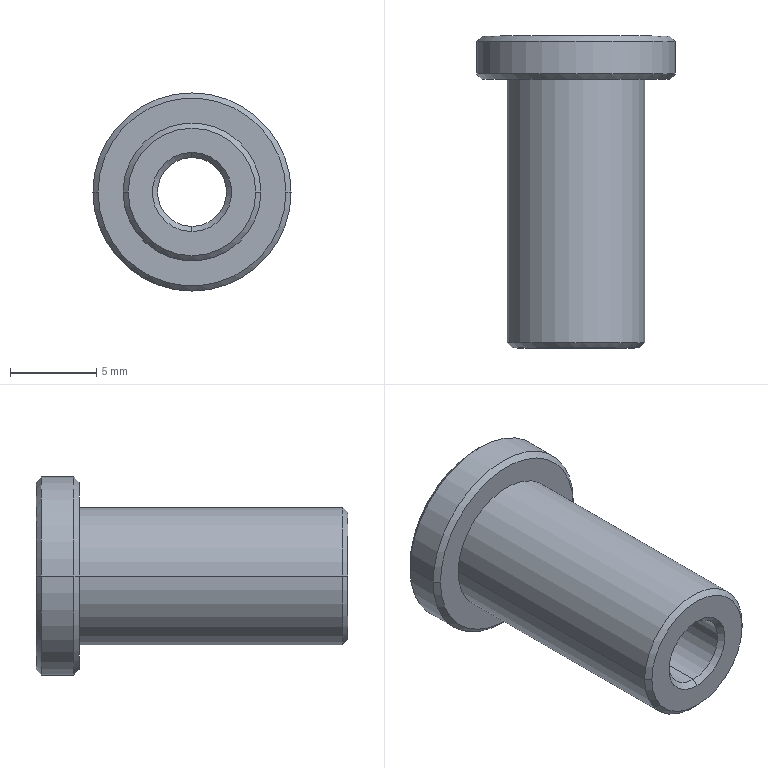Part | STEP file | 1 solid | 19 faces | box 11.5 x 18.1 x 11.5 mm | volume 810.877 mm3 | cone 10 | cylinder 6 | plane 3 | commonest cylinder face diameters 4 x2 8 x2 11.5 x2
STEP:
#1=CARTESIAN_POINT('',(0.,0.,0.));
#2=DIRECTION('',(0.,0.,1.));
#3=DIRECTION('',(1.,0.,0.));
#4=AXIS2_PLACEMENT_3D('',#1,#2,#3);
#5=CARTESIAN_POINT('',(3.7,0.,0.));
#6=VERTEX_POINT('',#5);
#7=CARTESIAN_POINT('',(-3.7,0.,0.));
#8=VERTEX_POINT('',#7);
#9=CARTESIAN_POINT('',(0.,0.,0.));
#10=DIRECTION('',(0.,-1.,0.));
#11=DIRECTION('',(1.,0.,0.));
#12=AXIS2_PLACEMENT_3D('',#9,#10,#11);
#13=CIRCLE('',#12,3.7);
#14=CARTESIAN_POINT('',(0.,0.3,0.));
#15=DIRECTION('',(0.,1.,0.));
#16=DIRECTION('',(-1.,0.,0.));
#17=AXIS2_PLACEMENT_3D('',#14,#15,#16);
#18=CONICAL_SURFACE('',#17,4.,0.7854);
#19=CARTESIAN_POINT('',(3.142,-0.3));
#20=DIRECTION('',(-1.,0.));
#21=VECTOR('',#20,1.);
#22=LINE('',#19,#21);
#23=(GEOMETRIC_REPRESENTATION_CONTEXT(2)PARAMETRIC_REPRESENTATION_CONTEXT()REPRESENTATION_CONTEXT('',''));
#24=DEFINITIONAL_REPRESENTATION('',(#22),#23);
#25=PCURVE('',#18,#24);
#26=CARTESIAN_POINT('',(-4.,0.,0.));
#27=DIRECTION('',(0.,-1.,0.));
#28=DIRECTION('',(1.,0.,0.));
#29=AXIS2_PLACEMENT_3D('',#26,#27,#28);
#30=PLANE('',#29);
#31=CARTESIAN_POINT('',(4.,0.));
#32=DIRECTION('',(1.,0.));
#33=AXIS2_PLACEMENT_2D('',#31,#32);
#34=CIRCLE('',#33,3.7);
#35=(GEOMETRIC_REPRESENTATION_CONTEXT(2)PARAMETRIC_REPRESENTATION_CONTEXT()REPRESENTATION_CONTEXT('',''));
#36=DEFINITIONAL_REPRESENTATION('',(#34),#35);
#37=PCURVE('',#30,#36);
#38=SURFACE_CURVE('',#13,(#25,#37),.PCURVE_S1.);
#39=EDGE_CURVE('',#6,#8,#38,.T.);
#40=ORIENTED_EDGE('',*,*,#39,.F.);
#41=CARTESIAN_POINT('',(4.,0.3,0.));
#42=VERTEX_POINT('',#41);
#43=CARTESIAN_POINT('',(4.,0.3,0.));
#44=DIRECTION('',(0.7071,0.7071,0.));
#45=VECTOR('',#44,1.);
#46=LINE('',#43,#45);
#47=CARTESIAN_POINT('',(3.142,0.));
#48=DIRECTION('',(0.,1.));
#49=VECTOR('',#48,1.);
#50=LINE('',#47,#49);
#51=(GEOMETRIC_REPRESENTATION_CONTEXT(2)PARAMETRIC_REPRESENTATION_CONTEXT()REPRESENTATION_CONTEXT('',''));
#52=DEFINITIONAL_REPRESENTATION('',(#50),#51);
#53=PCURVE('',#18,#52);
#54=CARTESIAN_POINT('',(0.,0.3,0.));
#55=DIRECTION('',(0.,1.,0.));
#56=DIRECTION('',(-1.,0.,0.));
#57=AXIS2_PLACEMENT_3D('',#54,#55,#56);
#58=CONICAL_SURFACE('',#57,4.,0.7854);
#59=CARTESIAN_POINT('',(3.142,0.));
#60=DIRECTION('',(0.,1.));
#61=VECTOR('',#60,1.);
#62=LINE('',#59,#61);
#63=(GEOMETRIC_REPRESENTATION_CONTEXT(2)PARAMETRIC_REPRESENTATION_CONTEXT()REPRESENTATION_CONTEXT('',''));
#64=DEFINITIONAL_REPRESENTATION('',(#62),#63);
#65=PCURVE('',#58,#64);
#66=SURFACE_CURVE('',#46,(#53,#65),.PCURVE_S1.);
#67=EDGE_CURVE('',#6,#42,#66,.T.);
#68=ORIENTED_EDGE('',*,*,#67,.T.);
#69=CARTESIAN_POINT('',(-4.,0.3,0.));
#70=VERTEX_POINT('',#69);
#71=CARTESIAN_POINT('',(0.,0.3,0.));
#72=DIRECTION('',(0.,1.,0.));
#73=DIRECTION('',(1.,0.,0.));
#74=AXIS2_PLACEMENT_3D('',#71,#72,#73);
#75=CIRCLE('',#74,4.);
#76=CARTESIAN_POINT('',(-3.142,0.));
#77=DIRECTION('',(1.,0.));
#78=VECTOR('',#77,1.);
#79=LINE('',#76,#78);
#80=(GEOMETRIC_REPRESENTATION_CONTEXT(2)PARAMETRIC_REPRESENTATION_CONTEXT()REPRESENTATION_CONTEXT('',''));
#81=DEFINITIONAL_REPRESENTATION('',(#79),#80);
#82=PCURVE('',#18,#81);
#83=CARTESIAN_POINT('',(0.,15.6,0.));
#84=DIRECTION('',(0.,1.,0.));
#85=DIRECTION('',(-1.,0.,0.));
#86=AXIS2_PLACEMENT_3D('',#83,#84,#85);
#87=CYLINDRICAL_SURFACE('',#86,4.);
#88=CARTESIAN_POINT('',(-3.142,-15.3));
#89=DIRECTION('',(1.,0.));
#90=VECTOR('',#89,1.);
#91=LINE('',#88,#90);
#92=(GEOMETRIC_REPRESENTATION_CONTEXT(2)PARAMETRIC_REPRESENTATION_CONTEXT()REPRESENTATION_CONTEXT('',''));
#93=DEFINITIONAL_REPRESENTATION('',(#91),#92);
#94=PCURVE('',#87,#93);
#95=SURFACE_CURVE('',#75,(#82,#94),.PCURVE_S1.);
#96=EDGE_CURVE('',#70,#42,#95,.T.);
#97=ORIENTED_EDGE('',*,*,#96,.F.);
#98=CARTESIAN_POINT('',(-4.,0.3,0.));
#99=DIRECTION('',(-0.7071,0.7071,0.));
#100=VECTOR('',#99,1.);
#101=LINE('',#98,#100);
#102=CARTESIAN_POINT('',(0.,0.));
#103=DIRECTION('',(0.,1.));
#104=VECTOR('',#103,1.);
#105=LINE('',#102,#104);
#106=(GEOMETRIC_REPRESENTATION_CONTEXT(2)PARAMETRIC_REPRESENTATION_CONTEXT()REPRESENTATION_CONTEXT('',''));
#107=DEFINITIONAL_REPRESENTATION('',(#105),#106);
#108=PCURVE('',#18,#107);
#109=CARTESIAN_POINT('',(6.283,0.));
#110=DIRECTION('',(0.,1.));
#111=VECTOR('',#110,1.);
#112=LINE('',#109,#111);
#113=(GEOMETRIC_REPRESENTATION_CONTEXT(2)PARAMETRIC_REPRESENTATION_CONTEXT()REPRESENTATION_CONTEXT('',''));
#114=DEFINITIONAL_REPRESENTATION('',(#112),#113);
#115=PCURVE('',#58,#114);
#116=SURFACE_CURVE('',#101,(#108,#115),.PCURVE_S1.);
#117=EDGE_CURVE('',#8,#70,#116,.T.);
#118=ORIENTED_EDGE('',*,*,#117,.F.);
#119=EDGE_LOOP('',(#40,#68,#97,#118));
#120=FACE_BOUND('',#119,.T.);
#121=ADVANCED_FACE('',(#120),#18,.T.);
#122=CARTESIAN_POINT('',(0.,0.3,-2.));
#123=VERTEX_POINT('',#122);
#124=CARTESIAN_POINT('',(0.,0.,-2.3));
#125=VERTEX_POINT('',#124);
#126=CARTESIAN_POINT('',(0.,0.,-2.3));
#127=DIRECTION('',(0.,-0.7071,-0.7071));
#128=VECTOR('',#127,1.);
#129=LINE('',#126,#128);
#130=CARTESIAN_POINT('',(0.,0.,0.));
#131=DIRECTION('',(0.,-1.,0.));
#132=DIRECTION('',(0.,0.,-1.));
#133=AXIS2_PLACEMENT_3D('',#130,#131,#132);
#134=CONICAL_SURFACE('',#133,2.3,0.7854);
#135=CARTESIAN_POINT('',(6.283,0.));
#136=DIRECTION('',(0.,1.));
#137=VECTOR('',#136,1.);
#138=LINE('',#135,#137);
#139=(GEOMETRIC_REPRESENTATION_CONTEXT(2)PARAMETRIC_REPRESENTATION_CONTEXT()REPRESENTATION_CONTEXT('',''));
#140=DEFINITIONAL_REPRESENTATION('',(#138),#139);
#141=PCURVE('',#134,#140);
#142=CARTESIAN_POINT('',(0.,0.,0.));
#143=DIRECTION('',(0.,-1.,0.));
#144=DIRECTION('',(0.,0.,-1.));
#145=AXIS2_PLACEMENT_3D('',#142,#143,#144);
#146=CONICAL_SURFACE('',#145,2.3,0.7854);
#147=CARTESIAN_POINT('',(0.,0.));
#148=DIRECTION('',(0.,1.));
#149=VECTOR('',#148,1.);
#150=LINE('',#147,#149);
#151=(GEOMETRIC_REPRESENTATION_CONTEXT(2)PARAMETRIC_REPRESENTATION_CONTEXT()REPRESENTATION_CONTEXT('',''));
#152=DEFINITIONAL_REPRESENTATION('',(#150),#151);
#153=PCURVE('',#146,#152);
#154=SURFACE_CURVE('',#129,(#141,#153),.PCURVE_S1.);
#155=EDGE_CURVE('',#123,#125,#154,.T.);
#156=ORIENTED_EDGE('',*,*,#155,.T.);
#157=CARTESIAN_POINT('',(0.,0.,2.3));
#158=VERTEX_POINT('',#157);
#159=CARTESIAN_POINT('',(0.,0.,0.));
#160=DIRECTION('',(0.,1.,0.));
#161=DIRECTION('',(1.,0.,0.));
#162=AXIS2_PLACEMENT_3D('',#159,#160,#161);
#163=CIRCLE('',#162,2.3);
#164=CARTESIAN_POINT('',(7.854,0.));
#165=DIRECTION('',(-1.,0.));
#166=VECTOR('',#165,1.);
#167=LINE('',#164,#166);
#168=(GEOMETRIC_REPRESENTATION_CONTEXT(2)PARAMETRIC_REPRESENTATION_CONTEXT()REPRESENTATION_CONTEXT('',''));
#169=DEFINITIONAL_REPRESENTATION('',(#167),#168);
#170=PCURVE('',#134,#169);
#171=CARTESIAN_POINT('',(6.3,0.));
#172=CARTESIAN_POINT('',(6.3,-3.984));
#173=CARTESIAN_POINT('',(2.85,-1.992));
#174=CARTESIAN_POINT('',(-0.6,0.));
#175=CARTESIAN_POINT('',(2.85,1.992));
#176=CARTESIAN_POINT('',(6.3,3.984));
#177=CARTESIAN_POINT('',(6.3,0.));
#178=(BOUNDED_CURVE()B_SPLINE_CURVE(2,(#171,#172,#173,#174,#175,#176,#177),.UNSPECIFIED.,.T.,.F.)B_SPLINE_CURVE_WITH_KNOTS((1,2,2,2,2,1),(-2.094,0.,2.094,4.189,6.283,8.378),.UNSPECIFIED.)CURVE()GEOMETRIC_REPRESENTATION_ITEM()RATIONAL_B_SPLINE_CURVE((1.,0.5,1.,0.5,1.,0.5,1.))REPRESENTATION_ITEM(''));
#179=(GEOMETRIC_REPRESENTATION_CONTEXT(2)PARAMETRIC_REPRESENTATION_CONTEXT()REPRESENTATION_CONTEXT('',''));
#180=DEFINITIONAL_REPRESENTATION('',(#178),#179);
#181=PCURVE('',#30,#180);
#182=SURFACE_CURVE('',#163,(#170,#181),.PCURVE_S1.);
#183=EDGE_CURVE('',#125,#158,#182,.T.);
#184=ORIENTED_EDGE('',*,*,#183,.T.);
#185=CARTESIAN_POINT('',(0.,0.3,2.));
#186=VERTEX_POINT('',#185);
#187=CARTESIAN_POINT('',(0.,0.,2.3));
#188=DIRECTION('',(0.,-0.7071,0.7071));
#189=VECTOR('',#188,1.);
#190=LINE('',#187,#189);
#191=CARTESIAN_POINT('',(3.142,0.));
#192=DIRECTION('',(0.,1.));
#193=VECTOR('',#192,1.);
#194=LINE('',#191,#193);
#195=(GEOMETRIC_REPRESENTATION_CONTEXT(2)PARAMETRIC_REPRESENTATION_CONTEXT()REPRESENTATION_CONTEXT('',''));
#196=DEFINITIONAL_REPRESENTATION('',(#194),#195);
#197=PCURVE('',#134,#196);
#198=CARTESIAN_POINT('',(3.142,0.));
#199=DIRECTION('',(0.,1.));
#200=VECTOR('',#199,1.);
#201=LINE('',#198,#200);
#202=(GEOMETRIC_REPRESENTATION_CONTEXT(2)PARAMETRIC_REPRESENTATION_CONTEXT()REPRESENTATION_CONTEXT('',''));
#203=DEFINITIONAL_REPRESENTATION('',(#201),#202);
#204=PCURVE('',#146,#203);
#205=SURFACE_CURVE('',#190,(#197,#204),.PCURVE_S1.);
#206=EDGE_CURVE('',#186,#158,#205,.T.);
#207=ORIENTED_EDGE('',*,*,#206,.F.);
#208=CARTESIAN_POINT('',(0.,0.3,0.));
#209=DIRECTION('',(0.,-1.,0.));
#210=DIRECTION('',(0.,0.,-1.));
#211=AXIS2_PLACEMENT_3D('',#208,#209,#210);
#212=CIRCLE('',#211,2.);
#213=CARTESIAN_POINT('',(0.,-0.3));
#214=DIRECTION('',(1.,0.));
#215=VECTOR('',#214,1.);
#216=LINE('',#213,#215);
#217=(GEOMETRIC_REPRESENTATION_CONTEXT(2)PARAMETRIC_REPRESENTATION_CONTEXT()REPRESENTATION_CONTEXT('',''));
#218=DEFINITIONAL_REPRESENTATION('',(#216),#217);
#219=PCURVE('',#134,#218);
#220=CARTESIAN_POINT('',(0.,18.1,0.));
#221=DIRECTION('',(0.,1.,0.));
#222=DIRECTION('',(0.,0.,1.));
#223=AXIS2_PLACEMENT_3D('',#220,#221,#222);
#224=CYLINDRICAL_SURFACE('',#223,2.);
#225=CARTESIAN_POINT('',(9.425,-17.8));
#226=DIRECTION('',(-1.,0.));
#227=VECTOR('',#226,1.);
#228=LINE('',#225,#227);
#229=(GEOMETRIC_REPRESENTATION_CONTEXT(2)PARAMETRIC_REPRESENTATION_CONTEXT()REPRESENTATION_CONTEXT('',''));
#230=DEFINITIONAL_REPRESENTATION('',(#228),#229);
#231=PCURVE('',#224,#230);
#232=SURFACE_CURVE('',#212,(#219,#231),.PCURVE_S1.);
#233=EDGE_CURVE('',#186,#123,#232,.T.);
#234=ORIENTED_EDGE('',*,*,#233,.T.);
#235=EDGE_LOOP('',(#156,#184,#207,#234));
#236=FACE_BOUND('',#235,.F.);
#237=ADVANCED_FACE('',(#236),#134,.F.);
#238=CARTESIAN_POINT('',(0.,17.8,2.));
#239=VERTEX_POINT('',#238);
#240=CARTESIAN_POINT('',(0.,18.1,2.3));
#241=VERTEX_POINT('',#240);
#242=CARTESIAN_POINT('',(0.,17.8,2.));
#243=DIRECTION('',(0.,0.7071,0.7071));
#244=VECTOR('',#243,1.);
#245=LINE('',#242,#244);
#246=CARTESIAN_POINT('',(0.,17.8,0.));
#247=DIRECTION('',(0.,1.,0.));
#248=DIRECTION('',(0.,0.,1.));
#249=AXIS2_PLACEMENT_3D('',#246,#247,#248);
#250=CONICAL_SURFACE('',#249,2.,0.7854);
#251=CARTESIAN_POINT('',(6.283,0.));
#252=DIRECTION('',(0.,1.));
#253=VECTOR('',#252,1.);
#254=LINE('',#251,#253);
#255=(GEOMETRIC_REPRESENTATION_CONTEXT(2)PARAMETRIC_REPRESENTATION_CONTEXT()REPRESENTATION_CONTEXT('',''));
#256=DEFINITIONAL_REPRESENTATION('',(#254),#255);
#257=PCURVE('',#250,#256);
#258=CARTESIAN_POINT('',(0.,17.8,0.));
#259=DIRECTION('',(0.,1.,0.));
#260=DIRECTION('',(0.,0.,1.));
#261=AXIS2_PLACEMENT_3D('',#258,#259,#260);
#262=CONICAL_SURFACE('',#261,2.,0.7854);
#263=CARTESIAN_POINT('',(0.,0.));
#264=DIRECTION('',(0.,1.));
#265=VECTOR('',#264,1.);
#266=LINE('',#263,#265);
#267=(GEOMETRIC_REPRESENTATION_CONTEXT(2)PARAMETRIC_REPRESENTATION_CONTEXT()REPRESENTATION_CONTEXT('',''));
#268=DEFINITIONAL_REPRESENTATION('',(#266),#267);
#269=PCURVE('',#262,#268);
#270=SURFACE_CURVE('',#245,(#257,#269),.PCURVE_S1.);
#271=EDGE_CURVE('',#239,#241,#270,.T.);
#272=ORIENTED_EDGE('',*,*,#271,.T.);
#273=CARTESIAN_POINT('',(0.,18.1,-2.3));
#274=VERTEX_POINT('',#273);
#275=CARTESIAN_POINT('',(0.,18.1,0.));
#276=DIRECTION('',(0.,-1.,0.));
#277=DIRECTION('',(-1.,0.,0.));
#278=AXIS2_PLACEMENT_3D('',#275,#276,#277);
#279=CIRCLE('',#278,2.3);
#280=CARTESIAN_POINT('',(10.996,0.3));
#281=DIRECTION('',(-1.,0.));
#282=VECTOR('',#281,1.);
#283=LINE('',#280,#282);
#284=(GEOMETRIC_REPRESENTATION_CONTEXT(2)PARAMETRIC_REPRESENTATION_CONTEXT()REPRESENTATION_CONTEXT('',''));
#285=DEFINITIONAL_REPRESENTATION('',(#283),#284);
#286=PCURVE('',#250,#285);
#287=CARTESIAN_POINT('',(0.,18.1,0.));
#288=DIRECTION('',(0.,1.,0.));
#289=DIRECTION('',(-1.,0.,0.));
#290=AXIS2_PLACEMENT_3D('',#287,#288,#289);
#291=PLANE('',#290);
#292=CARTESIAN_POINT('',(2.3,0.));
#293=CARTESIAN_POINT('',(2.3,-3.984));
#294=CARTESIAN_POINT('',(-1.15,-1.992));
#295=CARTESIAN_POINT('',(-4.6,0.));
#296=CARTESIAN_POINT('',(-1.15,1.992));
#297=CARTESIAN_POINT('',(2.3,3.984));
#298=CARTESIAN_POINT('',(2.3,0.));
#299=(BOUNDED_CURVE()B_SPLINE_CURVE(2,(#292,#293,#294,#295,#296,#297,#298),.UNSPECIFIED.,.T.,.F.)B_SPLINE_CURVE_WITH_KNOTS((1,2,2,2,2,1),(-2.094,0.,2.094,4.189,6.283,8.378),.UNSPECIFIED.)CURVE()GEOMETRIC_REPRESENTATION_ITEM()RATIONAL_B_SPLINE_CURVE((1.,0.5,1.,0.5,1.,0.5,1.))REPRESENTATION_ITEM(''));
#300=(GEOMETRIC_REPRESENTATION_CONTEXT(2)PARAMETRIC_REPRESENTATION_CONTEXT()REPRESENTATION_CONTEXT('',''));
#301=DEFINITIONAL_REPRESENTATION('',(#299),#300);
#302=PCURVE('',#291,#301);
#303=SURFACE_CURVE('',#279,(#286,#302),.PCURVE_S1.);
#304=EDGE_CURVE('',#241,#274,#303,.T.);
#305=ORIENTED_EDGE('',*,*,#304,.T.);
#306=CARTESIAN_POINT('',(0.,17.8,-2.));
#307=VERTEX_POINT('',#306);
#308=CARTESIAN_POINT('',(0.,17.8,-2.));
#309=DIRECTION('',(0.,0.7071,-0.7071));
#310=VECTOR('',#309,1.);
#311=LINE('',#308,#310);
#312=CARTESIAN_POINT('',(3.142,0.));
#313=DIRECTION('',(0.,1.));
#314=VECTOR('',#313,1.);
#315=LINE('',#312,#314);
#316=(GEOMETRIC_REPRESENTATION_CONTEXT(2)PARAMETRIC_REPRESENTATION_CONTEXT()REPRESENTATION_CONTEXT('',''));
#317=DEFINITIONAL_REPRESENTATION('',(#315),#316);
#318=PCURVE('',#250,#317);
#319=CARTESIAN_POINT('',(3.142,0.));
#320=DIRECTION('',(0.,1.));
#321=VECTOR('',#320,1.);
#322=LINE('',#319,#321);
#323=(GEOMETRIC_REPRESENTATION_CONTEXT(2)PARAMETRIC_REPRESENTATION_CONTEXT()REPRESENTATION_CONTEXT('',''));
#324=DEFINITIONAL_REPRESENTATION('',(#322),#323);
#325=PCURVE('',#262,#324);
#326=SURFACE_CURVE('',#311,(#318,#325),.PCURVE_S1.);
#327=EDGE_CURVE('',#307,#274,#326,.T.);
#328=ORIENTED_EDGE('',*,*,#327,.F.);
#329=CARTESIAN_POINT('',(0.,17.8,0.));
#330=DIRECTION('',(0.,1.,0.));
#331=DIRECTION('',(0.,0.,1.));
#332=AXIS2_PLACEMENT_3D('',#329,#330,#331);
#333=CIRCLE('',#332,2.);
#334=CARTESIAN_POINT('',(0.,0.));
#335=DIRECTION('',(1.,0.));
#336=VECTOR('',#335,1.);
#337=LINE('',#334,#336);
#338=(GEOMETRIC_REPRESENTATION_CONTEXT(2)PARAMETRIC_REPRESENTATION_CONTEXT()REPRESENTATION_CONTEXT('',''));
#339=DEFINITIONAL_REPRESENTATION('',(#337),#338);
#340=PCURVE('',#250,#339);
#341=CARTESIAN_POINT('',(0.,-0.3));
#342=DIRECTION('',(1.,0.));
#343=VECTOR('',#342,1.);
#344=LINE('',#341,#343);
#345=(GEOMETRIC_REPRESENTATION_CONTEXT(2)PARAMETRIC_REPRESENTATION_CONTEXT()REPRESENTATION_CONTEXT('',''));
#346=DEFINITIONAL_REPRESENTATION('',(#344),#345);
#347=PCURVE('',#224,#346);
#348=SURFACE_CURVE('',#333,(#340,#347),.PCURVE_S1.);
#349=EDGE_CURVE('',#307,#239,#348,.T.);
#350=ORIENTED_EDGE('',*,*,#349,.T.);
#351=EDGE_LOOP('',(#272,#305,#328,#350));
#352=FACE_BOUND('',#351,.F.);
#353=ADVANCED_FACE('',(#352),#250,.F.);
#354=CARTESIAN_POINT('',(-5.45,18.1,0.));
#355=VERTEX_POINT('',#354);
#356=CARTESIAN_POINT('',(5.45,18.1,0.));
#357=VERTEX_POINT('',#356);
#358=CARTESIAN_POINT('',(0.,18.1,0.));
#359=DIRECTION('',(0.,1.,0.));
#360=DIRECTION('',(-1.,0.,0.));
#361=AXIS2_PLACEMENT_3D('',#358,#359,#360);
#362=CIRCLE('',#361,5.45);
#363=CARTESIAN_POINT('',(0.,18.1,0.));
#364=DIRECTION('',(0.,-1.,0.));
#365=DIRECTION('',(1.,0.,0.));
#366=AXIS2_PLACEMENT_3D('',#363,#364,#365);
#367=CONICAL_SURFACE('',#366,5.45,0.7854);
#368=CARTESIAN_POINT('',(3.142,0.));
#369=DIRECTION('',(-1.,0.));
#370=VECTOR('',#369,1.);
#371=LINE('',#368,#370);
#372=(GEOMETRIC_REPRESENTATION_CONTEXT(2)PARAMETRIC_REPRESENTATION_CONTEXT()REPRESENTATION_CONTEXT('',''));
#373=DEFINITIONAL_REPRESENTATION('',(#371),#372);
#374=PCURVE('',#367,#373);
#375=CARTESIAN_POINT('',(0.,0.));
#376=DIRECTION('',(1.,0.));
#377=AXIS2_PLACEMENT_2D('',#375,#376);
#378=CIRCLE('',#377,5.45);
#379=(GEOMETRIC_REPRESENTATION_CONTEXT(2)PARAMETRIC_REPRESENTATION_CONTEXT()REPRESENTATION_CONTEXT('',''));
#380=DEFINITIONAL_REPRESENTATION('',(#378),#379);
#381=PCURVE('',#291,#380);
#382=SURFACE_CURVE('',#362,(#374,#381),.PCURVE_S1.);
#383=EDGE_CURVE('',#355,#357,#382,.T.);
#384=ORIENTED_EDGE('',*,*,#383,.F.);
#385=CARTESIAN_POINT('',(-5.75,17.8,0.));
#386=VERTEX_POINT('',#385);
#387=CARTESIAN_POINT('',(-5.45,18.1,0.));
#388=DIRECTION('',(-0.7071,-0.7071,0.));
#389=VECTOR('',#388,1.);
#390=LINE('',#387,#389);
#391=CARTESIAN_POINT('',(3.142,0.));
#392=DIRECTION('',(0.,1.));
#393=VECTOR('',#392,1.);
#394=LINE('',#391,#393);
#395=(GEOMETRIC_REPRESENTATION_CONTEXT(2)PARAMETRIC_REPRESENTATION_CONTEXT()REPRESENTATION_CONTEXT('',''));
#396=DEFINITIONAL_REPRESENTATION('',(#394),#395);
#397=PCURVE('',#367,#396);
#398=CARTESIAN_POINT('',(0.,18.1,0.));
#399=DIRECTION('',(0.,-1.,0.));
#400=DIRECTION('',(1.,0.,0.));
#401=AXIS2_PLACEMENT_3D('',#398,#399,#400);
#402=CONICAL_SURFACE('',#401,5.45,0.7854);
#403=CARTESIAN_POINT('',(3.142,0.));
#404=DIRECTION('',(0.,1.));
#405=VECTOR('',#404,1.);
#406=LINE('',#403,#405);
#407=(GEOMETRIC_REPRESENTATION_CONTEXT(2)PARAMETRIC_REPRESENTATION_CONTEXT()REPRESENTATION_CONTEXT('',''));
#408=DEFINITIONAL_REPRESENTATION('',(#406),#407);
#409=PCURVE('',#402,#408);
#410=SURFACE_CURVE('',#390,(#397,#409),.PCURVE_S1.);
#411=EDGE_CURVE('',#355,#386,#410,.T.);
#412=ORIENTED_EDGE('',*,*,#411,.T.);
#413=CARTESIAN_POINT('',(5.75,17.8,0.));
#414=VERTEX_POINT('',#413);
#415=CARTESIAN_POINT('',(0.,17.8,0.));
#416=DIRECTION('',(0.,-1.,0.));
#417=DIRECTION('',(-1.,0.,0.));
#418=AXIS2_PLACEMENT_3D('',#415,#416,#417);
#419=CIRCLE('',#418,5.75);
#420=CARTESIAN_POINT('',(-3.142,0.3));
#421=DIRECTION('',(1.,0.));
#422=VECTOR('',#421,1.);
#423=LINE('',#420,#422);
#424=(GEOMETRIC_REPRESENTATION_CONTEXT(2)PARAMETRIC_REPRESENTATION_CONTEXT()REPRESENTATION_CONTEXT('',''));
#425=DEFINITIONAL_REPRESENTATION('',(#423),#424);
#426=PCURVE('',#367,#425);
#427=CARTESIAN_POINT('',(0.,18.1,0.));
#428=DIRECTION('',(0.,-1.,0.));
#429=DIRECTION('',(1.,0.,0.));
#430=AXIS2_PLACEMENT_3D('',#427,#428,#429);
#431=CYLINDRICAL_SURFACE('',#430,5.75);
#432=CARTESIAN_POINT('',(-3.142,0.3));
#433=DIRECTION('',(1.,0.));
#434=VECTOR('',#433,1.);
#435=LINE('',#432,#434);
#436=(GEOMETRIC_REPRESENTATION_CONTEXT(2)PARAMETRIC_REPRESENTATION_CONTEXT()REPRESENTATION_CONTEXT('',''));
#437=DEFINITIONAL_REPRESENTATION('',(#435),#436);
#438=PCURVE('',#431,#437);
#439=SURFACE_CURVE('',#419,(#426,#438),.PCURVE_S1.);
#440=EDGE_CURVE('',#414,#386,#439,.T.);
#441=ORIENTED_EDGE('',*,*,#440,.F.);
#442=CARTESIAN_POINT('',(5.45,18.1,0.));
#443=DIRECTION('',(0.7071,-0.7071,0.));
#444=VECTOR('',#443,1.);
#445=LINE('',#442,#444);
#446=CARTESIAN_POINT('',(0.,0.));
#447=DIRECTION('',(0.,1.));
#448=VECTOR('',#447,1.);
#449=LINE('',#446,#448);
#450=(GEOMETRIC_REPRESENTATION_CONTEXT(2)PARAMETRIC_REPRESENTATION_CONTEXT()REPRESENTATION_CONTEXT('',''));
#451=DEFINITIONAL_REPRESENTATION('',(#449),#450);
#452=PCURVE('',#367,#451);
#453=CARTESIAN_POINT('',(6.283,0.));
#454=DIRECTION('',(0.,1.));
#455=VECTOR('',#454,1.);
#456=LINE('',#453,#455);
#457=(GEOMETRIC_REPRESENTATION_CONTEXT(2)PARAMETRIC_REPRESENTATION_CONTEXT()REPRESENTATION_CONTEXT('',''));
#458=DEFINITIONAL_REPRESENTATION('',(#456),#457);
#459=PCURVE('',#402,#458);
#460=SURFACE_CURVE('',#445,(#452,#459),.PCURVE_S1.);
#461=EDGE_CURVE('',#357,#414,#460,.T.);
#462=ORIENTED_EDGE('',*,*,#461,.F.);
#463=EDGE_LOOP('',(#384,#412,#441,#462));
#464=FACE_BOUND('',#463,.T.);
#465=ADVANCED_FACE('',(#464),#367,.T.);
#466=CARTESIAN_POINT('',(5.45,15.6,0.));
#467=VERTEX_POINT('',#466);
#468=CARTESIAN_POINT('',(-5.45,15.6,0.));
#469=VERTEX_POINT('',#468);
#470=CARTESIAN_POINT('',(0.,15.6,0.));
#471=DIRECTION('',(0.,-1.,0.));
#472=DIRECTION('',(-1.,0.,0.));
#473=AXIS2_PLACEMENT_3D('',#470,#471,#472);
#474=CIRCLE('',#473,5.45);
#475=CARTESIAN_POINT('',(0.,15.9,0.));
#476=DIRECTION('',(0.,1.,0.));
#477=DIRECTION('',(-1.,0.,0.));
#478=AXIS2_PLACEMENT_3D('',#475,#476,#477);
#479=CONICAL_SURFACE('',#478,5.75,0.7854);
#480=CARTESIAN_POINT('',(6.283,-0.3));
#481=DIRECTION('',(-1.,0.));
#482=VECTOR('',#481,1.);
#483=LINE('',#480,#482);
#484=(GEOMETRIC_REPRESENTATION_CONTEXT(2)PARAMETRIC_REPRESENTATION_CONTEXT()REPRESENTATION_CONTEXT('',''));
#485=DEFINITIONAL_REPRESENTATION('',(#483),#484);
#486=PCURVE('',#479,#485);
#487=CARTESIAN_POINT('',(0.,15.6,0.));
#488=DIRECTION('',(0.,1.,0.));
#489=DIRECTION('',(-1.,0.,0.));
#490=AXIS2_PLACEMENT_3D('',#487,#488,#489);
#491=PLANE('',#490);
#492=CARTESIAN_POINT('',(5.45,0.));
#493=CARTESIAN_POINT('',(5.45,-9.44));
#494=CARTESIAN_POINT('',(-2.725,-4.72));
#495=CARTESIAN_POINT('',(-10.9,0.));
#496=CARTESIAN_POINT('',(-2.725,4.72));
#497=CARTESIAN_POINT('',(5.45,9.44));
#498=CARTESIAN_POINT('',(5.45,0.));
#499=(BOUNDED_CURVE()B_SPLINE_CURVE(2,(#492,#493,#494,#495,#496,#497,#498),.UNSPECIFIED.,.T.,.F.)B_SPLINE_CURVE_WITH_KNOTS((1,2,2,2,2,1),(-2.094,0.,2.094,4.189,6.283,8.378),.UNSPECIFIED.)CURVE()GEOMETRIC_REPRESENTATION_ITEM()RATIONAL_B_SPLINE_CURVE((1.,0.5,1.,0.5,1.,0.5,1.))REPRESENTATION_ITEM(''));
#500=(GEOMETRIC_REPRESENTATION_CONTEXT(2)PARAMETRIC_REPRESENTATION_CONTEXT()REPRESENTATION_CONTEXT('',''));
#501=DEFINITIONAL_REPRESENTATION('',(#499),#500);
#502=PCURVE('',#491,#501);
#503=SURFACE_CURVE('',#474,(#486,#502),.PCURVE_S1.);
#504=EDGE_CURVE('',#467,#469,#503,.T.);
#505=ORIENTED_EDGE('',*,*,#504,.F.);
#506=CARTESIAN_POINT('',(5.75,15.9,0.));
#507=VERTEX_POINT('',#506);
#508=CARTESIAN_POINT('',(5.75,15.9,0.));
#509=DIRECTION('',(0.7071,0.7071,0.));
#510=VECTOR('',#509,1.);
#511=LINE('',#508,#510);
#512=CARTESIAN_POINT('',(3.142,0.));
#513=DIRECTION('',(0.,1.));
#514=VECTOR('',#513,1.);
#515=LINE('',#512,#514);
#516=(GEOMETRIC_REPRESENTATION_CONTEXT(2)PARAMETRIC_REPRESENTATION_CONTEXT()REPRESENTATION_CONTEXT('',''));
#517=DEFINITIONAL_REPRESENTATION('',(#515),#516);
#518=PCURVE('',#479,#517);
#519=CARTESIAN_POINT('',(0.,15.9,0.));
#520=DIRECTION('',(0.,1.,0.));
#521=DIRECTION('',(-1.,0.,0.));
#522=AXIS2_PLACEMENT_3D('',#519,#520,#521);
#523=CONICAL_SURFACE('',#522,5.75,0.7854);
#524=CARTESIAN_POINT('',(3.142,0.));
#525=DIRECTION('',(0.,1.));
#526=VECTOR('',#525,1.);
#527=LINE('',#524,#526);
#528=(GEOMETRIC_REPRESENTATION_CONTEXT(2)PARAMETRIC_REPRESENTATION_CONTEXT()REPRESENTATION_CONTEXT('',''));
#529=DEFINITIONAL_REPRESENTATION('',(#527),#528);
#530=PCURVE('',#523,#529);
#531=SURFACE_CURVE('',#511,(#518,#530),.PCURVE_S1.);
#532=EDGE_CURVE('',#467,#507,#531,.T.);
#533=ORIENTED_EDGE('',*,*,#532,.T.);
#534=CARTESIAN_POINT('',(-5.75,15.9,0.));
#535=VERTEX_POINT('',#534);
#536=CARTESIAN_POINT('',(0.,15.9,0.));
#537=DIRECTION('',(0.,1.,0.));
#538=DIRECTION('',(-1.,0.,0.));
#539=AXIS2_PLACEMENT_3D('',#536,#537,#538);
#540=CIRCLE('',#539,5.75);
#541=CARTESIAN_POINT('',(0.,0.));
#542=DIRECTION('',(1.,0.));
#543=VECTOR('',#542,1.);
#544=LINE('',#541,#543);
#545=(GEOMETRIC_REPRESENTATION_CONTEXT(2)PARAMETRIC_REPRESENTATION_CONTEXT()REPRESENTATION_CONTEXT('',''));
#546=DEFINITIONAL_REPRESENTATION('',(#544),#545);
#547=PCURVE('',#479,#546);
#548=CARTESIAN_POINT('',(3.142,2.2));
#549=DIRECTION('',(-1.,0.));
#550=VECTOR('',#549,1.);
#551=LINE('',#548,#550);
#552=(GEOMETRIC_REPRESENTATION_CONTEXT(2)PARAMETRIC_REPRESENTATION_CONTEXT()REPRESENTATION_CONTEXT('',''));
#553=DEFINITIONAL_REPRESENTATION('',(#551),#552);
#554=PCURVE('',#431,#553);
#555=SURFACE_CURVE('',#540,(#547,#554),.PCURVE_S1.);
#556=EDGE_CURVE('',#535,#507,#555,.T.);
#557=ORIENTED_EDGE('',*,*,#556,.F.);
#558=CARTESIAN_POINT('',(-5.75,15.9,0.));
#559=DIRECTION('',(-0.7071,0.7071,0.));
#560=VECTOR('',#559,1.);
#561=LINE('',#558,#560);
#562=CARTESIAN_POINT('',(0.,0.));
#563=DIRECTION('',(0.,1.));
#564=VECTOR('',#563,1.);
#565=LINE('',#562,#564);
#566=(GEOMETRIC_REPRESENTATION_CONTEXT(2)PARAMETRIC_REPRESENTATION_CONTEXT()REPRESENTATION_CONTEXT('',''));
#567=DEFINITIONAL_REPRESENTATION('',(#565),#566);
#568=PCURVE('',#479,#567);
#569=CARTESIAN_POINT('',(6.283,0.));
#570=DIRECTION('',(0.,1.));
#571=VECTOR('',#570,1.);
#572=LINE('',#569,#571);
#573=(GEOMETRIC_REPRESENTATION_CONTEXT(2)PARAMETRIC_REPRESENTATION_CONTEXT()REPRESENTATION_CONTEXT('',''));
#574=DEFINITIONAL_REPRESENTATION('',(#572),#573);
#575=PCURVE('',#523,#574);
#576=SURFACE_CURVE('',#561,(#568,#575),.PCURVE_S1.);
#577=EDGE_CURVE('',#469,#535,#576,.T.);
#578=ORIENTED_EDGE('',*,*,#577,.F.);
#579=EDGE_LOOP('',(#505,#533,#557,#578));
#580=FACE_BOUND('',#579,.T.);
#581=ADVANCED_FACE('',(#580),#479,.T.);
#582=CARTESIAN_POINT('',(0.,18.1,2.));
#583=DIRECTION('',(0.,1.,0.));
#584=VECTOR('',#583,1.);
#585=LINE('',#582,#584);
#586=CARTESIAN_POINT('',(6.283,0.));
#587=DIRECTION('',(0.,1.));
#588=VECTOR('',#587,1.);
#589=LINE('',#586,#588);
#590=(GEOMETRIC_REPRESENTATION_CONTEXT(2)PARAMETRIC_REPRESENTATION_CONTEXT()REPRESENTATION_CONTEXT('',''));
#591=DEFINITIONAL_REPRESENTATION('',(#589),#590);
#592=PCURVE('',#224,#591);
#593=CARTESIAN_POINT('',(0.,18.1,0.));
#594=DIRECTION('',(0.,1.,0.));
#595=DIRECTION('',(0.,0.,1.));
#596=AXIS2_PLACEMENT_3D('',#593,#594,#595);
#597=CYLINDRICAL_SURFACE('',#596,2.);
#598=CARTESIAN_POINT('',(0.,0.));
#599=DIRECTION('',(0.,1.));
#600=VECTOR('',#599,1.);
#601=LINE('',#598,#600);
#602=(GEOMETRIC_REPRESENTATION_CONTEXT(2)PARAMETRIC_REPRESENTATION_CONTEXT()REPRESENTATION_CONTEXT('',''));
#603=DEFINITIONAL_REPRESENTATION('',(#601),#602);
#604=PCURVE('',#597,#603);
#605=SURFACE_CURVE('',#585,(#592,#604),.PCURVE_S1.);
#606=EDGE_CURVE('',#186,#239,#605,.T.);
#607=ORIENTED_EDGE('',*,*,#606,.T.);
#608=ORIENTED_EDGE('',*,*,#349,.F.);
#609=CARTESIAN_POINT('',(0.,18.1,-2.));
#610=DIRECTION('',(0.,1.,0.));
#611=VECTOR('',#610,1.);
#612=LINE('',#609,#611);
#613=CARTESIAN_POINT('',(3.142,0.));
#614=DIRECTION('',(0.,1.));
#615=VECTOR('',#614,1.);
#616=LINE('',#613,#615);
#617=(GEOMETRIC_REPRESENTATION_CONTEXT(2)PARAMETRIC_REPRESENTATION_CONTEXT()REPRESENTATION_CONTEXT('',''));
#618=DEFINITIONAL_REPRESENTATION('',(#616),#617);
#619=PCURVE('',#224,#618);
#620=CARTESIAN_POINT('',(3.142,0.));
#621=DIRECTION('',(0.,1.));
#622=VECTOR('',#621,1.);
#623=LINE('',#620,#622);
#624=(GEOMETRIC_REPRESENTATION_CONTEXT(2)PARAMETRIC_REPRESENTATION_CONTEXT()REPRESENTATION_CONTEXT('',''));
#625=DEFINITIONAL_REPRESENTATION('',(#623),#624);
#626=PCURVE('',#597,#625);
#627=SURFACE_CURVE('',#612,(#619,#626),.PCURVE_S1.);
#628=EDGE_CURVE('',#123,#307,#627,.T.);
#629=ORIENTED_EDGE('',*,*,#628,.F.);
#630=ORIENTED_EDGE('',*,*,#233,.F.);
#631=EDGE_LOOP('',(#607,#608,#629,#630));
#632=FACE_BOUND('',#631,.F.);
#633=ADVANCED_FACE('',(#632),#224,.F.);
#634=ORIENTED_EDGE('',*,*,#440,.T.);
#635=CARTESIAN_POINT('',(-5.75,18.1,0.));
#636=DIRECTION('',(0.,-1.,0.));
#637=VECTOR('',#636,1.);
#638=LINE('',#635,#637);
#639=CARTESIAN_POINT('',(3.142,0.));
#640=DIRECTION('',(0.,1.));
#641=VECTOR('',#640,1.);
#642=LINE('',#639,#641);
#643=(GEOMETRIC_REPRESENTATION_CONTEXT(2)PARAMETRIC_REPRESENTATION_CONTEXT()REPRESENTATION_CONTEXT('',''));
#644=DEFINITIONAL_REPRESENTATION('',(#642),#643);
#645=PCURVE('',#431,#644);
#646=CARTESIAN_POINT('',(0.,18.1,0.));
#647=DIRECTION('',(0.,-1.,0.));
#648=DIRECTION('',(1.,0.,0.));
#649=AXIS2_PLACEMENT_3D('',#646,#647,#648);
#650=CYLINDRICAL_SURFACE('',#649,5.75);
#651=CARTESIAN_POINT('',(3.142,0.));
#652=DIRECTION('',(0.,1.));
#653=VECTOR('',#652,1.);
#654=LINE('',#651,#653);
#655=(GEOMETRIC_REPRESENTATION_CONTEXT(2)PARAMETRIC_REPRESENTATION_CONTEXT()REPRESENTATION_CONTEXT('',''));
#656=DEFINITIONAL_REPRESENTATION('',(#654),#655);
#657=PCURVE('',#650,#656);
#658=SURFACE_CURVE('',#638,(#645,#657),.PCURVE_S1.);
#659=EDGE_CURVE('',#386,#535,#658,.T.);
#660=ORIENTED_EDGE('',*,*,#659,.T.);
#661=ORIENTED_EDGE('',*,*,#556,.T.);
#662=CARTESIAN_POINT('',(5.75,18.1,0.));
#663=DIRECTION('',(0.,-1.,0.));
#664=VECTOR('',#663,1.);
#665=LINE('',#662,#664);
#666=CARTESIAN_POINT('',(0.,0.));
#667=DIRECTION('',(0.,1.));
#668=VECTOR('',#667,1.);
#669=LINE('',#666,#668);
#670=(GEOMETRIC_REPRESENTATION_CONTEXT(2)PARAMETRIC_REPRESENTATION_CONTEXT()REPRESENTATION_CONTEXT('',''));
#671=DEFINITIONAL_REPRESENTATION('',(#669),#670);
#672=PCURVE('',#431,#671);
#673=CARTESIAN_POINT('',(6.283,0.));
#674=DIRECTION('',(0.,1.));
#675=VECTOR('',#674,1.);
#676=LINE('',#673,#675);
#677=(GEOMETRIC_REPRESENTATION_CONTEXT(2)PARAMETRIC_REPRESENTATION_CONTEXT()REPRESENTATION_CONTEXT('',''));
#678=DEFINITIONAL_REPRESENTATION('',(#676),#677);
#679=PCURVE('',#650,#678);
#680=SURFACE_CURVE('',#665,(#672,#679),.PCURVE_S1.);
#681=EDGE_CURVE('',#414,#507,#680,.T.);
#682=ORIENTED_EDGE('',*,*,#681,.F.);
#683=EDGE_LOOP('',(#634,#660,#661,#682));
#684=FACE_BOUND('',#683,.T.);
#685=ADVANCED_FACE('',(#684),#431,.T.);
#686=ORIENTED_EDGE('',*,*,#96,.T.);
#687=CARTESIAN_POINT('',(4.,15.6,0.));
#688=VERTEX_POINT('',#687);
#689=CARTESIAN_POINT('',(4.,15.6,0.));
#690=DIRECTION('',(0.,1.,0.));
#691=VECTOR('',#690,1.);
#692=LINE('',#689,#691);
#693=CARTESIAN_POINT('',(3.142,0.));
#694=DIRECTION('',(0.,1.));
#695=VECTOR('',#694,1.);
#696=LINE('',#693,#695);
#697=(GEOMETRIC_REPRESENTATION_CONTEXT(2)PARAMETRIC_REPRESENTATION_CONTEXT()REPRESENTATION_CONTEXT('',''));
#698=DEFINITIONAL_REPRESENTATION('',(#696),#697);
#699=PCURVE('',#87,#698);
#700=CARTESIAN_POINT('',(0.,15.6,0.));
#701=DIRECTION('',(0.,1.,0.));
#702=DIRECTION('',(-1.,0.,0.));
#703=AXIS2_PLACEMENT_3D('',#700,#701,#702);
#704=CYLINDRICAL_SURFACE('',#703,4.);
#705=CARTESIAN_POINT('',(3.142,0.));
#706=DIRECTION('',(0.,1.));
#707=VECTOR('',#706,1.);
#708=LINE('',#705,#707);
#709=(GEOMETRIC_REPRESENTATION_CONTEXT(2)PARAMETRIC_REPRESENTATION_CONTEXT()REPRESENTATION_CONTEXT('',''));
#710=DEFINITIONAL_REPRESENTATION('',(#708),#709);
#711=PCURVE('',#704,#710);
#712=SURFACE_CURVE('',#692,(#699,#711),.PCURVE_S1.);
#713=EDGE_CURVE('',#42,#688,#712,.T.);
#714=ORIENTED_EDGE('',*,*,#713,.T.);
#715=CARTESIAN_POINT('',(-4.,15.6,0.));
#716=VERTEX_POINT('',#715);
#717=CARTESIAN_POINT('',(0.,15.6,0.));
#718=DIRECTION('',(0.,1.,0.));
#719=DIRECTION('',(-1.,0.,0.));
#720=AXIS2_PLACEMENT_3D('',#717,#718,#719);
#721=CIRCLE('',#720,4.);
#722=CARTESIAN_POINT('',(0.,0.));
#723=DIRECTION('',(1.,0.));
#724=VECTOR('',#723,1.);
#725=LINE('',#722,#724);
#726=(GEOMETRIC_REPRESENTATION_CONTEXT(2)PARAMETRIC_REPRESENTATION_CONTEXT()REPRESENTATION_CONTEXT('',''));
#727=DEFINITIONAL_REPRESENTATION('',(#725),#726);
#728=PCURVE('',#87,#727);
#729=CARTESIAN_POINT('',(0.,0.));
#730=DIRECTION('',(1.,0.));
#731=AXIS2_PLACEMENT_2D('',#729,#730);
#732=CIRCLE('',#731,4.);
#733=(GEOMETRIC_REPRESENTATION_CONTEXT(2)PARAMETRIC_REPRESENTATION_CONTEXT()REPRESENTATION_CONTEXT('',''));
#734=DEFINITIONAL_REPRESENTATION('',(#732),#733);
#735=PCURVE('',#491,#734);
#736=SURFACE_CURVE('',#721,(#728,#735),.PCURVE_S1.);
#737=EDGE_CURVE('',#716,#688,#736,.T.);
#738=ORIENTED_EDGE('',*,*,#737,.F.);
#739=CARTESIAN_POINT('',(-4.,15.6,0.));
#740=DIRECTION('',(0.,1.,0.));
#741=VECTOR('',#740,1.);
#742=LINE('',#739,#741);
#743=CARTESIAN_POINT('',(0.,0.));
#744=DIRECTION('',(0.,1.));
#745=VECTOR('',#744,1.);
#746=LINE('',#743,#745);
#747=(GEOMETRIC_REPRESENTATION_CONTEXT(2)PARAMETRIC_REPRESENTATION_CONTEXT()REPRESENTATION_CONTEXT('',''));
#748=DEFINITIONAL_REPRESENTATION('',(#746),#747);
#749=PCURVE('',#87,#748);
#750=CARTESIAN_POINT('',(6.283,0.));
#751=DIRECTION('',(0.,1.));
#752=VECTOR('',#751,1.);
#753=LINE('',#750,#752);
#754=(GEOMETRIC_REPRESENTATION_CONTEXT(2)PARAMETRIC_REPRESENTATION_CONTEXT()REPRESENTATION_CONTEXT('',''));
#755=DEFINITIONAL_REPRESENTATION('',(#753),#754);
#756=PCURVE('',#704,#755);
#757=SURFACE_CURVE('',#742,(#749,#756),.PCURVE_S1.);
#758=EDGE_CURVE('',#70,#716,#757,.T.);
#759=ORIENTED_EDGE('',*,*,#758,.F.);
#760=EDGE_LOOP('',(#686,#714,#738,#759));
#761=FACE_BOUND('',#760,.T.);
#762=ADVANCED_FACE('',(#761),#87,.T.);
#763=ORIENTED_EDGE('',*,*,#713,.F.);
#764=CARTESIAN_POINT('',(0.,0.3,0.));
#765=DIRECTION('',(0.,1.,0.));
#766=DIRECTION('',(1.,0.,0.));
#767=AXIS2_PLACEMENT_3D('',#764,#765,#766);
#768=CIRCLE('',#767,4.);
#769=CARTESIAN_POINT('',(3.142,-15.3));
#770=DIRECTION('',(1.,0.));
#771=VECTOR('',#770,1.);
#772=LINE('',#769,#771);
#773=(GEOMETRIC_REPRESENTATION_CONTEXT(2)PARAMETRIC_REPRESENTATION_CONTEXT()REPRESENTATION_CONTEXT('',''));
#774=DEFINITIONAL_REPRESENTATION('',(#772),#773);
#775=PCURVE('',#704,#774);
#776=CARTESIAN_POINT('',(3.142,0.));
#777=DIRECTION('',(1.,0.));
#778=VECTOR('',#777,1.);
#779=LINE('',#776,#778);
#780=(GEOMETRIC_REPRESENTATION_CONTEXT(2)PARAMETRIC_REPRESENTATION_CONTEXT()REPRESENTATION_CONTEXT('',''));
#781=DEFINITIONAL_REPRESENTATION('',(#779),#780);
#782=PCURVE('',#58,#781);
#783=SURFACE_CURVE('',#768,(#775,#782),.PCURVE_S1.);
#784=EDGE_CURVE('',#42,#70,#783,.T.);
#785=ORIENTED_EDGE('',*,*,#784,.T.);
#786=ORIENTED_EDGE('',*,*,#758,.T.);
#787=CARTESIAN_POINT('',(0.,15.6,0.));
#788=DIRECTION('',(0.,1.,0.));
#789=DIRECTION('',(-1.,0.,0.));
#790=AXIS2_PLACEMENT_3D('',#787,#788,#789);
#791=CIRCLE('',#790,4.);
#792=CARTESIAN_POINT('',(0.,0.));
#793=DIRECTION('',(1.,0.));
#794=VECTOR('',#793,1.);
#795=LINE('',#792,#794);
#796=(GEOMETRIC_REPRESENTATION_CONTEXT(2)PARAMETRIC_REPRESENTATION_CONTEXT()REPRESENTATION_CONTEXT('',''));
#797=DEFINITIONAL_REPRESENTATION('',(#795),#796);
#798=PCURVE('',#704,#797);
#799=CARTESIAN_POINT('',(0.,0.));
#800=DIRECTION('',(1.,0.));
#801=AXIS2_PLACEMENT_2D('',#799,#800);
#802=CIRCLE('',#801,4.);
#803=(GEOMETRIC_REPRESENTATION_CONTEXT(2)PARAMETRIC_REPRESENTATION_CONTEXT()REPRESENTATION_CONTEXT('',''));
#804=DEFINITIONAL_REPRESENTATION('',(#802),#803);
#805=PCURVE('',#491,#804);
#806=SURFACE_CURVE('',#791,(#798,#805),.PCURVE_S1.);
#807=EDGE_CURVE('',#688,#716,#806,.T.);
#808=ORIENTED_EDGE('',*,*,#807,.F.);
#809=EDGE_LOOP('',(#763,#785,#786,#808));
#810=FACE_BOUND('',#809,.T.);
#811=ADVANCED_FACE('',(#810),#704,.T.);
#812=ORIENTED_EDGE('',*,*,#183,.T.);
#813=CARTESIAN_POINT('',(0.,0.,0.));
#814=DIRECTION('',(0.,1.,0.));
#815=DIRECTION('',(1.,0.,0.));
#816=AXIS2_PLACEMENT_3D('',#813,#814,#815);
#817=CIRCLE('',#816,2.3);
#818=CARTESIAN_POINT('',(6.3,0.));
#819=CARTESIAN_POINT('',(6.3,-3.984));
#820=CARTESIAN_POINT('',(2.85,-1.992));
#821=CARTESIAN_POINT('',(-0.6,0.));
#822=CARTESIAN_POINT('',(2.85,1.992));
#823=CARTESIAN_POINT('',(6.3,3.984));
#824=CARTESIAN_POINT('',(6.3,0.));
#825=(BOUNDED_CURVE()B_SPLINE_CURVE(2,(#818,#819,#820,#821,#822,#823,#824),.UNSPECIFIED.,.T.,.F.)B_SPLINE_CURVE_WITH_KNOTS((1,2,2,2,2,1),(-2.094,0.,2.094,4.189,6.283,8.378),.UNSPECIFIED.)CURVE()GEOMETRIC_REPRESENTATION_ITEM()RATIONAL_B_SPLINE_CURVE((1.,0.5,1.,0.5,1.,0.5,1.))REPRESENTATION_ITEM(''));
#826=(GEOMETRIC_REPRESENTATION_CONTEXT(2)PARAMETRIC_REPRESENTATION_CONTEXT()REPRESENTATION_CONTEXT('',''));
#827=DEFINITIONAL_REPRESENTATION('',(#825),#826);
#828=PCURVE('',#30,#827);
#829=CARTESIAN_POINT('',(7.854,0.));
#830=DIRECTION('',(-1.,0.));
#831=VECTOR('',#830,1.);
#832=LINE('',#829,#831);
#833=(GEOMETRIC_REPRESENTATION_CONTEXT(2)PARAMETRIC_REPRESENTATION_CONTEXT()REPRESENTATION_CONTEXT('',''));
#834=DEFINITIONAL_REPRESENTATION('',(#832),#833);
#835=PCURVE('',#146,#834);
#836=SURFACE_CURVE('',#817,(#828,#835),.PCURVE_S1.);
#837=EDGE_CURVE('',#158,#125,#836,.T.);
#838=ORIENTED_EDGE('',*,*,#837,.T.);
#839=EDGE_LOOP('',(#812,#838));
#840=FACE_BOUND('',#839,.T.);
#841=CARTESIAN_POINT('',(0.,0.,0.));
#842=DIRECTION('',(0.,-1.,0.));
#843=DIRECTION('',(1.,0.,0.));
#844=AXIS2_PLACEMENT_3D('',#841,#842,#843);
#845=CIRCLE('',#844,3.7);
#846=CARTESIAN_POINT('',(4.,0.));
#847=DIRECTION('',(1.,0.));
#848=AXIS2_PLACEMENT_2D('',#846,#847);
#849=CIRCLE('',#848,3.7);
#850=(GEOMETRIC_REPRESENTATION_CONTEXT(2)PARAMETRIC_REPRESENTATION_CONTEXT()REPRESENTATION_CONTEXT('',''));
#851=DEFINITIONAL_REPRESENTATION('',(#849),#850);
#852=PCURVE('',#30,#851);
#853=CARTESIAN_POINT('',(9.425,-0.3));
#854=DIRECTION('',(-1.,0.));
#855=VECTOR('',#854,1.);
#856=LINE('',#853,#855);
#857=(GEOMETRIC_REPRESENTATION_CONTEXT(2)PARAMETRIC_REPRESENTATION_CONTEXT()REPRESENTATION_CONTEXT('',''));
#858=DEFINITIONAL_REPRESENTATION('',(#856),#857);
#859=PCURVE('',#58,#858);
#860=SURFACE_CURVE('',#845,(#852,#859),.PCURVE_S1.);
#861=EDGE_CURVE('',#8,#6,#860,.T.);
#862=ORIENTED_EDGE('',*,*,#861,.T.);
#863=ORIENTED_EDGE('',*,*,#39,.T.);
#864=EDGE_LOOP('',(#862,#863));
#865=FACE_BOUND('',#864,.T.);
#866=ADVANCED_FACE('',(#840,#865),#30,.T.);
#867=ORIENTED_EDGE('',*,*,#659,.F.);
#868=CARTESIAN_POINT('',(0.,17.8,0.));
#869=DIRECTION('',(0.,-1.,0.));
#870=DIRECTION('',(-1.,0.,0.));
#871=AXIS2_PLACEMENT_3D('',#868,#869,#870);
#872=CIRCLE('',#871,5.75);
#873=CARTESIAN_POINT('',(3.142,0.3));
#874=DIRECTION('',(1.,0.));
#875=VECTOR('',#874,1.);
#876=LINE('',#873,#875);
#877=(GEOMETRIC_REPRESENTATION_CONTEXT(2)PARAMETRIC_REPRESENTATION_CONTEXT()REPRESENTATION_CONTEXT('',''));
#878=DEFINITIONAL_REPRESENTATION('',(#876),#877);
#879=PCURVE('',#650,#878);
#880=CARTESIAN_POINT('',(3.142,0.3));
#881=DIRECTION('',(1.,0.));
#882=VECTOR('',#881,1.);
#883=LINE('',#880,#882);
#884=(GEOMETRIC_REPRESENTATION_CONTEXT(2)PARAMETRIC_REPRESENTATION_CONTEXT()REPRESENTATION_CONTEXT('',''));
#885=DEFINITIONAL_REPRESENTATION('',(#883),#884);
#886=PCURVE('',#402,#885);
#887=SURFACE_CURVE('',#872,(#879,#886),.PCURVE_S1.);
#888=EDGE_CURVE('',#386,#414,#887,.T.);
#889=ORIENTED_EDGE('',*,*,#888,.T.);
#890=ORIENTED_EDGE('',*,*,#681,.T.);
#891=CARTESIAN_POINT('',(0.,15.9,0.));
#892=DIRECTION('',(0.,1.,0.));
#893=DIRECTION('',(-1.,0.,0.));
#894=AXIS2_PLACEMENT_3D('',#891,#892,#893);
#895=CIRCLE('',#894,5.75);
#896=CARTESIAN_POINT('',(9.425,2.2));
#897=DIRECTION('',(-1.,0.));
#898=VECTOR('',#897,1.);
#899=LINE('',#896,#898);
#900=(GEOMETRIC_REPRESENTATION_CONTEXT(2)PARAMETRIC_REPRESENTATION_CONTEXT()REPRESENTATION_CONTEXT('',''));
#901=DEFINITIONAL_REPRESENTATION('',(#899),#900);
#902=PCURVE('',#650,#901);
#903=CARTESIAN_POINT('',(0.,0.));
#904=DIRECTION('',(1.,0.));
#905=VECTOR('',#904,1.);
#906=LINE('',#903,#905);
#907=(GEOMETRIC_REPRESENTATION_CONTEXT(2)PARAMETRIC_REPRESENTATION_CONTEXT()REPRESENTATION_CONTEXT('',''));
#908=DEFINITIONAL_REPRESENTATION('',(#906),#907);
#909=PCURVE('',#523,#908);
#910=SURFACE_CURVE('',#895,(#902,#909),.PCURVE_S1.);
#911=EDGE_CURVE('',#507,#535,#910,.T.);
#912=ORIENTED_EDGE('',*,*,#911,.T.);
#913=EDGE_LOOP('',(#867,#889,#890,#912));
#914=FACE_BOUND('',#913,.T.);
#915=ADVANCED_FACE('',(#914),#650,.T.);
#916=CARTESIAN_POINT('',(0.,18.1,0.));
#917=DIRECTION('',(0.,1.,0.));
#918=DIRECTION('',(-1.,0.,0.));
#919=AXIS2_PLACEMENT_3D('',#916,#917,#918);
#920=CIRCLE('',#919,5.45);
#921=CARTESIAN_POINT('',(0.,0.));
#922=DIRECTION('',(1.,0.));
#923=AXIS2_PLACEMENT_2D('',#921,#922);
#924=CIRCLE('',#923,5.45);
#925=(GEOMETRIC_REPRESENTATION_CONTEXT(2)PARAMETRIC_REPRESENTATION_CONTEXT()REPRESENTATION_CONTEXT('',''));
#926=DEFINITIONAL_REPRESENTATION('',(#924),#925);
#927=PCURVE('',#291,#926);
#928=CARTESIAN_POINT('',(9.425,0.));
#929=DIRECTION('',(-1.,0.));
#930=VECTOR('',#929,1.);
#931=LINE('',#928,#930);
#932=(GEOMETRIC_REPRESENTATION_CONTEXT(2)PARAMETRIC_REPRESENTATION_CONTEXT()REPRESENTATION_CONTEXT('',''));
#933=DEFINITIONAL_REPRESENTATION('',(#931),#932);
#934=PCURVE('',#402,#933);
#935=SURFACE_CURVE('',#920,(#927,#934),.PCURVE_S1.);
#936=EDGE_CURVE('',#357,#355,#935,.T.);
#937=ORIENTED_EDGE('',*,*,#936,.T.);
#938=ORIENTED_EDGE('',*,*,#383,.T.);
#939=EDGE_LOOP('',(#937,#938));
#940=FACE_BOUND('',#939,.T.);
#941=ORIENTED_EDGE('',*,*,#304,.T.);
#942=CARTESIAN_POINT('',(0.,18.1,0.));
#943=DIRECTION('',(0.,-1.,0.));
#944=DIRECTION('',(-1.,0.,0.));
#945=AXIS2_PLACEMENT_3D('',#942,#943,#944);
#946=CIRCLE('',#945,2.3);
#947=CARTESIAN_POINT('',(2.3,0.));
#948=CARTESIAN_POINT('',(2.3,-3.984));
#949=CARTESIAN_POINT('',(-1.15,-1.992));
#950=CARTESIAN_POINT('',(-4.6,0.));
#951=CARTESIAN_POINT('',(-1.15,1.992));
#952=CARTESIAN_POINT('',(2.3,3.984));
#953=CARTESIAN_POINT('',(2.3,0.));
#954=(BOUNDED_CURVE()B_SPLINE_CURVE(2,(#947,#948,#949,#950,#951,#952,#953),.UNSPECIFIED.,.T.,.F.)B_SPLINE_CURVE_WITH_KNOTS((1,2,2,2,2,1),(-2.094,0.,2.094,4.189,6.283,8.378),.UNSPECIFIED.)CURVE()GEOMETRIC_REPRESENTATION_ITEM()RATIONAL_B_SPLINE_CURVE((1.,0.5,1.,0.5,1.,0.5,1.))REPRESENTATION_ITEM(''));
#955=(GEOMETRIC_REPRESENTATION_CONTEXT(2)PARAMETRIC_REPRESENTATION_CONTEXT()REPRESENTATION_CONTEXT('',''));
#956=DEFINITIONAL_REPRESENTATION('',(#954),#955);
#957=PCURVE('',#291,#956);
#958=CARTESIAN_POINT('',(4.712,0.3));
#959=DIRECTION('',(-1.,0.));
#960=VECTOR('',#959,1.);
#961=LINE('',#958,#960);
#962=(GEOMETRIC_REPRESENTATION_CONTEXT(2)PARAMETRIC_REPRESENTATION_CONTEXT()REPRESENTATION_CONTEXT('',''));
#963=DEFINITIONAL_REPRESENTATION('',(#961),#962);
#964=PCURVE('',#262,#963);
#965=SURFACE_CURVE('',#946,(#957,#964),.PCURVE_S1.);
#966=EDGE_CURVE('',#274,#241,#965,.T.);
#967=ORIENTED_EDGE('',*,*,#966,.T.);
#968=EDGE_LOOP('',(#941,#967));
#969=FACE_BOUND('',#968,.T.);
#970=ADVANCED_FACE('',(#940,#969),#291,.T.);
#971=CARTESIAN_POINT('',(0.,15.6,0.));
#972=DIRECTION('',(0.,-1.,0.));
#973=DIRECTION('',(-1.,0.,0.));
#974=AXIS2_PLACEMENT_3D('',#971,#972,#973);
#975=CIRCLE('',#974,5.45);
#976=CARTESIAN_POINT('',(5.45,0.));
#977=CARTESIAN_POINT('',(5.45,-9.44));
#978=CARTESIAN_POINT('',(-2.725,-4.72));
#979=CARTESIAN_POINT('',(-10.9,0.));
#980=CARTESIAN_POINT('',(-2.725,4.72));
#981=CARTESIAN_POINT('',(5.45,9.44));
#982=CARTESIAN_POINT('',(5.45,0.));
#983=(BOUNDED_CURVE()B_SPLINE_CURVE(2,(#976,#977,#978,#979,#980,#981,#982),.UNSPECIFIED.,.T.,.F.)B_SPLINE_CURVE_WITH_KNOTS((1,2,2,2,2,1),(-2.094,0.,2.094,4.189,6.283,8.378),.UNSPECIFIED.)CURVE()GEOMETRIC_REPRESENTATION_ITEM()RATIONAL_B_SPLINE_CURVE((1.,0.5,1.,0.5,1.,0.5,1.))REPRESENTATION_ITEM(''));
#984=(GEOMETRIC_REPRESENTATION_CONTEXT(2)PARAMETRIC_REPRESENTATION_CONTEXT()REPRESENTATION_CONTEXT('',''));
#985=DEFINITIONAL_REPRESENTATION('',(#983),#984);
#986=PCURVE('',#491,#985);
#987=CARTESIAN_POINT('',(6.283,-0.3));
#988=DIRECTION('',(-1.,0.));
#989=VECTOR('',#988,1.);
#990=LINE('',#987,#989);
#991=(GEOMETRIC_REPRESENTATION_CONTEXT(2)PARAMETRIC_REPRESENTATION_CONTEXT()REPRESENTATION_CONTEXT('',''));
#992=DEFINITIONAL_REPRESENTATION('',(#990),#991);
#993=PCURVE('',#523,#992);
#994=SURFACE_CURVE('',#975,(#986,#993),.PCURVE_S1.);
#995=EDGE_CURVE('',#469,#467,#994,.T.);
#996=ORIENTED_EDGE('',*,*,#995,.T.);
#997=ORIENTED_EDGE('',*,*,#504,.T.);
#998=EDGE_LOOP('',(#996,#997));
#999=FACE_BOUND('',#998,.T.);
#1000=ORIENTED_EDGE('',*,*,#737,.T.);
#1001=ORIENTED_EDGE('',*,*,#807,.T.);
#1002=EDGE_LOOP('',(#1000,#1001));
#1003=FACE_BOUND('',#1002,.T.);
#1004=ADVANCED_FACE('',(#999,#1003),#491,.F.);
#1005=CARTESIAN_POINT('',(0.,17.8,0.));
#1006=DIRECTION('',(0.,1.,0.));
#1007=DIRECTION('',(0.,0.,1.));
#1008=AXIS2_PLACEMENT_3D('',#1005,#1006,#1007);
#1009=CIRCLE('',#1008,2.);
#1010=CARTESIAN_POINT('',(0.,-0.3));
#1011=DIRECTION('',(1.,0.));
#1012=VECTOR('',#1011,1.);
#1013=LINE('',#1010,#1012);
#1014=(GEOMETRIC_REPRESENTATION_CONTEXT(2)PARAMETRIC_REPRESENTATION_CONTEXT()REPRESENTATION_CONTEXT('',''));
#1015=DEFINITIONAL_REPRESENTATION('',(#1013),#1014);
#1016=PCURVE('',#597,#1015);
#1017=CARTESIAN_POINT('',(0.,0.));
#1018=DIRECTION('',(1.,0.));
#1019=VECTOR('',#1018,1.);
#1020=LINE('',#1017,#1019);
#1021=(GEOMETRIC_REPRESENTATION_CONTEXT(2)PARAMETRIC_REPRESENTATION_CONTEXT()REPRESENTATION_CONTEXT('',''));
#1022=DEFINITIONAL_REPRESENTATION('',(#1020),#1021);
#1023=PCURVE('',#262,#1022);
#1024=SURFACE_CURVE('',#1009,(#1016,#1023),.PCURVE_S1.);
#1025=EDGE_CURVE('',#239,#307,#1024,.T.);
#1026=ORIENTED_EDGE('',*,*,#1025,.F.);
#1027=ORIENTED_EDGE('',*,*,#606,.F.);
#1028=CARTESIAN_POINT('',(0.,0.3,0.));
#1029=DIRECTION('',(0.,-1.,0.));
#1030=DIRECTION('',(0.,0.,-1.));
#1031=AXIS2_PLACEMENT_3D('',#1028,#1029,#1030);
#1032=CIRCLE('',#1031,2.);
#1033=CARTESIAN_POINT('',(3.142,-17.8));
#1034=DIRECTION('',(-1.,0.));
#1035=VECTOR('',#1034,1.);
#1036=LINE('',#1033,#1035);
#1037=(GEOMETRIC_REPRESENTATION_CONTEXT(2)PARAMETRIC_REPRESENTATION_CONTEXT()REPRESENTATION_CONTEXT('',''));
#1038=DEFINITIONAL_REPRESENTATION('',(#1036),#1037);
#1039=PCURVE('',#597,#1038);
#1040=CARTESIAN_POINT('',(0.,-0.3));
#1041=DIRECTION('',(1.,0.));
#1042=VECTOR('',#1041,1.);
#1043=LINE('',#1040,#1042);
#1044=(GEOMETRIC_REPRESENTATION_CONTEXT(2)PARAMETRIC_REPRESENTATION_CONTEXT()REPRESENTATION_CONTEXT('',''));
#1045=DEFINITIONAL_REPRESENTATION('',(#1043),#1044);
#1046=PCURVE('',#146,#1045);
#1047=SURFACE_CURVE('',#1032,(#1039,#1046),.PCURVE_S1.);
#1048=EDGE_CURVE('',#123,#186,#1047,.T.);
#1049=ORIENTED_EDGE('',*,*,#1048,.F.);
#1050=ORIENTED_EDGE('',*,*,#628,.T.);
#1051=EDGE_LOOP('',(#1026,#1027,#1049,#1050));
#1052=FACE_BOUND('',#1051,.F.);
#1053=ADVANCED_FACE('',(#1052),#597,.F.);
#1054=ORIENTED_EDGE('',*,*,#532,.F.);
#1055=ORIENTED_EDGE('',*,*,#995,.F.);
#1056=ORIENTED_EDGE('',*,*,#577,.T.);
#1057=ORIENTED_EDGE('',*,*,#911,.F.);
#1058=EDGE_LOOP('',(#1054,#1055,#1056,#1057));
#1059=FACE_BOUND('',#1058,.T.);
#1060=ADVANCED_FACE('',(#1059),#523,.T.);
#1061=ORIENTED_EDGE('',*,*,#411,.F.);
#1062=ORIENTED_EDGE('',*,*,#936,.F.);
#1063=ORIENTED_EDGE('',*,*,#461,.T.);
#1064=ORIENTED_EDGE('',*,*,#888,.F.);
#1065=EDGE_LOOP('',(#1061,#1062,#1063,#1064));
#1066=FACE_BOUND('',#1065,.T.);
#1067=ADVANCED_FACE('',(#1066),#402,.T.);
#1068=ORIENTED_EDGE('',*,*,#966,.T.);
#1069=ORIENTED_EDGE('',*,*,#271,.F.);
#1070=ORIENTED_EDGE('',*,*,#1025,.T.);
#1071=ORIENTED_EDGE('',*,*,#327,.T.);
#1072=EDGE_LOOP('',(#1068,#1069,#1070,#1071));
#1073=FACE_BOUND('',#1072,.F.);
#1074=ADVANCED_FACE('',(#1073),#262,.F.);
#1075=ORIENTED_EDGE('',*,*,#837,.T.);
#1076=ORIENTED_EDGE('',*,*,#155,.F.);
#1077=ORIENTED_EDGE('',*,*,#1048,.T.);
#1078=ORIENTED_EDGE('',*,*,#206,.T.);
#1079=EDGE_LOOP('',(#1075,#1076,#1077,#1078));
#1080=FACE_BOUND('',#1079,.F.);
#1081=ADVANCED_FACE('',(#1080),#146,.F.);
#1082=ORIENTED_EDGE('',*,*,#67,.F.);
#1083=ORIENTED_EDGE('',*,*,#861,.F.);
#1084=ORIENTED_EDGE('',*,*,#117,.T.);
#1085=ORIENTED_EDGE('',*,*,#784,.F.);
#1086=EDGE_LOOP('',(#1082,#1083,#1084,#1085));
#1087=FACE_BOUND('',#1086,.T.);
#1088=ADVANCED_FACE('',(#1087),#58,.T.);
#1089=CLOSED_SHELL('',(#121,#237,#353,#465,#581,#633,#685,#762,#811,#866,#915,#970,#1004,#1053,#1060,#1067,#1074,#1081,#1088));
#1090=MANIFOLD_SOLID_BREP('',#1089);
#1091=(LENGTH_UNIT()NAMED_UNIT(*)SI_UNIT(.MILLI.,.METRE.));
#1092=UNCERTAINTY_MEASURE_WITH_UNIT(LENGTH_MEASURE(0.0000001),#1091,'','');
#1093=(NAMED_UNIT(*)PLANE_ANGLE_UNIT()SI_UNIT($,.RADIAN.));
#1094=(NAMED_UNIT(*)SI_UNIT($,.STERADIAN.)SOLID_ANGLE_UNIT());
#1095=(GEOMETRIC_REPRESENTATION_CONTEXT(3)GLOBAL_UNCERTAINTY_ASSIGNED_CONTEXT((#1092))GLOBAL_UNIT_ASSIGNED_CONTEXT((#1091,#1093,#1094))REPRESENTATION_CONTEXT('',''));
#1096=ADVANCED_BREP_SHAPE_REPRESENTATION('',(#4,#1090),#1095);